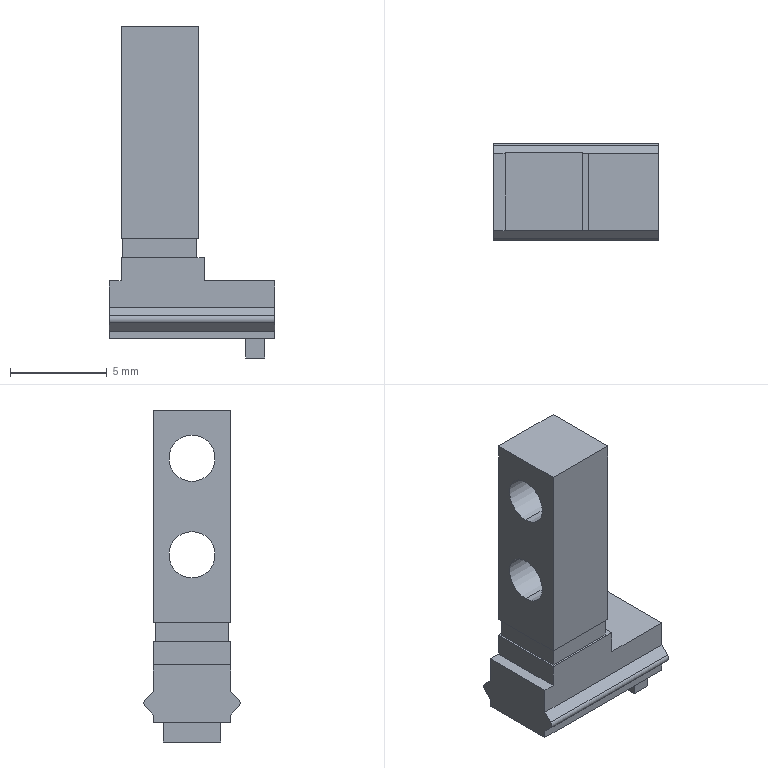Part | STEP file | MHZ2-6D2_Finger(0).stp | 1 solid | 37 faces | box 8.55 x 5 x 17.2 mm | volume 286.489 mm3 | plane 31 | cylinder 6 | commonest cylinder face diameters 2.4 x4 0.5 x2
STEP:
#1=CARTESIAN_POINT('',(-10.,0.,9.9));
#2=VERTEX_POINT('',#1);
#3=CARTESIAN_POINT('',(-10.,0.,7.5));
#4=VERTEX_POINT('',#3);
#5=CARTESIAN_POINT('',(-10.,0.,8.7));
#6=DIRECTION('',(1.,0.,0.));
#7=DIRECTION('',(0.,0.,-1.));
#8=AXIS2_PLACEMENT_3D('',#5,#6,#7);
#9=CIRCLE('',#8,1.2);
#10=EDGE_CURVE('',#2,#4,#9,.T.);
#11=ORIENTED_EDGE('',*,*,#10,.F.);
#12=CARTESIAN_POINT('',(-6.,0.,9.9));
#13=VERTEX_POINT('',#12);
#14=CARTESIAN_POINT('',(-6.,0.,9.9));
#15=DIRECTION('',(1.,0.,0.));
#16=VECTOR('',#15,1000.);
#17=LINE('',#14,#16);
#18=EDGE_CURVE('',#2,#13,#17,.T.);
#19=ORIENTED_EDGE('',*,*,#18,.T.);
#20=CARTESIAN_POINT('',(-6.,0.,7.5));
#21=VERTEX_POINT('',#20);
#22=CARTESIAN_POINT('',(-6.,0.,8.7));
#23=DIRECTION('',(1.,0.,0.));
#24=DIRECTION('',(0.,0.,-1.));
#25=AXIS2_PLACEMENT_3D('',#22,#23,#24);
#26=CIRCLE('',#25,1.2);
#27=EDGE_CURVE('',#13,#21,#26,.T.);
#28=ORIENTED_EDGE('',*,*,#27,.T.);
#29=CARTESIAN_POINT('',(-6.,0.,7.5));
#30=DIRECTION('',(1.,0.,0.));
#31=VECTOR('',#30,1000.);
#32=LINE('',#29,#31);
#33=EDGE_CURVE('',#4,#21,#32,.T.);
#34=ORIENTED_EDGE('',*,*,#33,.F.);
#35=EDGE_LOOP('',(#11,#19,#28,#34));
#36=FACE_OUTER_BOUND('',#35,.T.);
#37=CARTESIAN_POINT('',(-6.,0.,8.7));
#38=DIRECTION('',(1.,0.,0.));
#39=DIRECTION('',(0.,0.,-1.));
#40=AXIS2_PLACEMENT_3D('',#37,#38,#39);
#41=CYLINDRICAL_SURFACE('',#40,1.2);
#42=ADVANCED_FACE('',(#36),#41,.F.);
#43=CARTESIAN_POINT('',(-10.,0.,14.9));
#44=VERTEX_POINT('',#43);
#45=CARTESIAN_POINT('',(-10.,0.,12.5));
#46=VERTEX_POINT('',#45);
#47=CARTESIAN_POINT('',(-10.,0.,13.7));
#48=DIRECTION('',(1.,0.,0.));
#49=DIRECTION('',(0.,0.,-1.));
#50=AXIS2_PLACEMENT_3D('',#47,#48,#49);
#51=CIRCLE('',#50,1.2);
#52=EDGE_CURVE('',#44,#46,#51,.T.);
#53=ORIENTED_EDGE('',*,*,#52,.F.);
#54=CARTESIAN_POINT('',(-6.,0.,14.9));
#55=VERTEX_POINT('',#54);
#56=CARTESIAN_POINT('',(-6.,0.,14.9));
#57=DIRECTION('',(1.,0.,0.));
#58=VECTOR('',#57,1000.);
#59=LINE('',#56,#58);
#60=EDGE_CURVE('',#44,#55,#59,.T.);
#61=ORIENTED_EDGE('',*,*,#60,.T.);
#62=CARTESIAN_POINT('',(-6.,0.,12.5));
#63=VERTEX_POINT('',#62);
#64=CARTESIAN_POINT('',(-6.,0.,13.7));
#65=DIRECTION('',(1.,0.,0.));
#66=DIRECTION('',(0.,0.,-1.));
#67=AXIS2_PLACEMENT_3D('',#64,#65,#66);
#68=CIRCLE('',#67,1.2);
#69=EDGE_CURVE('',#55,#63,#68,.T.);
#70=ORIENTED_EDGE('',*,*,#69,.T.);
#71=CARTESIAN_POINT('',(-6.,0.,12.5));
#72=DIRECTION('',(1.,0.,0.));
#73=VECTOR('',#72,1000.);
#74=LINE('',#71,#73);
#75=EDGE_CURVE('',#46,#63,#74,.T.);
#76=ORIENTED_EDGE('',*,*,#75,.F.);
#77=EDGE_LOOP('',(#53,#61,#70,#76));
#78=FACE_OUTER_BOUND('',#77,.T.);
#79=CARTESIAN_POINT('',(-6.,0.,13.7));
#80=DIRECTION('',(1.,0.,0.));
#81=DIRECTION('',(0.,0.,-1.));
#82=AXIS2_PLACEMENT_3D('',#79,#80,#81);
#83=CYLINDRICAL_SURFACE('',#82,1.2);
#84=ADVANCED_FACE('',(#78),#83,.F.);
#85=CARTESIAN_POINT('',(-10.6,-2.,1.604));
#86=VERTEX_POINT('',#85);
#87=CARTESIAN_POINT('',(-10.6,-2.,3.));
#88=VERTEX_POINT('',#87);
#89=CARTESIAN_POINT('',(-10.6,-2.,0.));
#90=DIRECTION('',(0.,0.,1.));
#91=VECTOR('',#90,1000.);
#92=LINE('',#89,#91);
#93=EDGE_CURVE('',#86,#88,#92,.T.);
#94=ORIENTED_EDGE('',*,*,#93,.F.);
#95=CARTESIAN_POINT('',(-2.05,-2.,1.604));
#96=VERTEX_POINT('',#95);
#97=CARTESIAN_POINT('',(-10.6,-2.,1.604));
#98=DIRECTION('',(1.,0.,0.));
#99=VECTOR('',#98,1000.);
#100=LINE('',#97,#99);
#101=EDGE_CURVE('',#86,#96,#100,.T.);
#102=ORIENTED_EDGE('',*,*,#101,.T.);
#103=CARTESIAN_POINT('',(-2.05,-2.,3.));
#104=VERTEX_POINT('',#103);
#105=CARTESIAN_POINT('',(-2.05,-2.,3.));
#106=DIRECTION('',(0.,0.,-1.));
#107=VECTOR('',#106,1000.);
#108=LINE('',#105,#107);
#109=EDGE_CURVE('',#104,#96,#108,.T.);
#110=ORIENTED_EDGE('',*,*,#109,.F.);
#111=CARTESIAN_POINT('',(-5.7,-2.,3.));
#112=VERTEX_POINT('',#111);
#113=CARTESIAN_POINT('',(-5.7,-2.,3.));
#114=DIRECTION('',(1.,0.,0.));
#115=VECTOR('',#114,1000.);
#116=LINE('',#113,#115);
#117=EDGE_CURVE('',#112,#104,#116,.T.);
#118=ORIENTED_EDGE('',*,*,#117,.F.);
#119=CARTESIAN_POINT('',(-5.7,-2.,4.2));
#120=VERTEX_POINT('',#119);
#121=CARTESIAN_POINT('',(-5.7,-2.,4.2));
#122=DIRECTION('',(0.,0.,-1.));
#123=VECTOR('',#122,1000.);
#124=LINE('',#121,#123);
#125=EDGE_CURVE('',#120,#112,#124,.T.);
#126=ORIENTED_EDGE('',*,*,#125,.F.);
#127=CARTESIAN_POINT('',(-10.,-2.,4.2));
#128=VERTEX_POINT('',#127);
#129=CARTESIAN_POINT('',(-6.1,-2.,4.2));
#130=DIRECTION('',(1.,0.,0.));
#131=VECTOR('',#130,1000.);
#132=LINE('',#129,#131);
#133=EDGE_CURVE('',#128,#120,#132,.T.);
#134=ORIENTED_EDGE('',*,*,#133,.F.);
#135=CARTESIAN_POINT('',(-10.,-2.,3.));
#136=VERTEX_POINT('',#135);
#137=CARTESIAN_POINT('',(-10.,-2.,3.));
#138=DIRECTION('',(0.,0.,1.));
#139=VECTOR('',#138,1000.);
#140=LINE('',#137,#139);
#141=EDGE_CURVE('',#136,#128,#140,.T.);
#142=ORIENTED_EDGE('',*,*,#141,.F.);
#143=CARTESIAN_POINT('',(-10.6,-2.,3.));
#144=DIRECTION('',(1.,0.,0.));
#145=VECTOR('',#144,1000.);
#146=LINE('',#143,#145);
#147=EDGE_CURVE('',#88,#136,#146,.T.);
#148=ORIENTED_EDGE('',*,*,#147,.F.);
#149=EDGE_LOOP('',(#94,#102,#110,#118,#126,#134,#142,#148));
#150=FACE_OUTER_BOUND('',#149,.T.);
#151=CARTESIAN_POINT('',(0.,-2.,0.));
#152=DIRECTION('',(0.,1.,0.));
#153=DIRECTION('',(1.,0.,0.));
#154=AXIS2_PLACEMENT_3D('',#151,#152,#153);
#155=PLANE('',#154);
#156=ADVANCED_FACE('',(#150),#155,.F.);
#157=CARTESIAN_POINT('',(-10.6,2.,1.604));
#158=VERTEX_POINT('',#157);
#159=CARTESIAN_POINT('',(-2.05,2.,1.604));
#160=VERTEX_POINT('',#159);
#161=CARTESIAN_POINT('',(-10.6,2.,1.604));
#162=DIRECTION('',(1.,0.,0.));
#163=VECTOR('',#162,1000.);
#164=LINE('',#161,#163);
#165=EDGE_CURVE('',#158,#160,#164,.T.);
#166=ORIENTED_EDGE('',*,*,#165,.F.);
#167=CARTESIAN_POINT('',(-10.6,2.,3.));
#168=VERTEX_POINT('',#167);
#169=CARTESIAN_POINT('',(-10.6,2.,0.));
#170=DIRECTION('',(0.,0.,1.));
#171=VECTOR('',#170,1000.);
#172=LINE('',#169,#171);
#173=EDGE_CURVE('',#158,#168,#172,.T.);
#174=ORIENTED_EDGE('',*,*,#173,.T.);
#175=CARTESIAN_POINT('',(-10.,2.,3.));
#176=VERTEX_POINT('',#175);
#177=CARTESIAN_POINT('',(-10.6,2.,3.));
#178=DIRECTION('',(1.,0.,0.));
#179=VECTOR('',#178,1000.);
#180=LINE('',#177,#179);
#181=EDGE_CURVE('',#168,#176,#180,.T.);
#182=ORIENTED_EDGE('',*,*,#181,.T.);
#183=CARTESIAN_POINT('',(-10.,2.,4.2));
#184=VERTEX_POINT('',#183);
#185=CARTESIAN_POINT('',(-10.,2.,3.));
#186=DIRECTION('',(0.,0.,1.));
#187=VECTOR('',#186,1000.);
#188=LINE('',#185,#187);
#189=EDGE_CURVE('',#176,#184,#188,.T.);
#190=ORIENTED_EDGE('',*,*,#189,.T.);
#191=CARTESIAN_POINT('',(-5.7,2.,4.2));
#192=VERTEX_POINT('',#191);
#193=CARTESIAN_POINT('',(-10.,2.,4.2));
#194=DIRECTION('',(1.,0.,0.));
#195=VECTOR('',#194,1000.);
#196=LINE('',#193,#195);
#197=EDGE_CURVE('',#184,#192,#196,.T.);
#198=ORIENTED_EDGE('',*,*,#197,.T.);
#199=CARTESIAN_POINT('',(-5.7,2.,3.));
#200=VERTEX_POINT('',#199);
#201=CARTESIAN_POINT('',(-5.7,2.,4.2));
#202=DIRECTION('',(0.,0.,-1.));
#203=VECTOR('',#202,1000.);
#204=LINE('',#201,#203);
#205=EDGE_CURVE('',#192,#200,#204,.T.);
#206=ORIENTED_EDGE('',*,*,#205,.T.);
#207=CARTESIAN_POINT('',(-2.05,2.,3.));
#208=VERTEX_POINT('',#207);
#209=CARTESIAN_POINT('',(-5.7,2.,3.));
#210=DIRECTION('',(1.,0.,0.));
#211=VECTOR('',#210,1000.);
#212=LINE('',#209,#211);
#213=EDGE_CURVE('',#200,#208,#212,.T.);
#214=ORIENTED_EDGE('',*,*,#213,.T.);
#215=CARTESIAN_POINT('',(-2.05,2.,3.));
#216=DIRECTION('',(0.,0.,-1.));
#217=VECTOR('',#216,1000.);
#218=LINE('',#215,#217);
#219=EDGE_CURVE('',#208,#160,#218,.T.);
#220=ORIENTED_EDGE('',*,*,#219,.T.);
#221=EDGE_LOOP('',(#166,#174,#182,#190,#198,#206,#214,#220));
#222=FACE_OUTER_BOUND('',#221,.T.);
#223=CARTESIAN_POINT('',(0.,2.,0.));
#224=DIRECTION('',(0.,1.,0.));
#225=DIRECTION('',(1.,0.,0.));
#226=AXIS2_PLACEMENT_3D('',#223,#224,#225);
#227=PLANE('',#226);
#228=ADVANCED_FACE('',(#222),#227,.T.);
#229=CARTESIAN_POINT('',(-2.05,-2.,0.));
#230=VERTEX_POINT('',#229);
#231=CARTESIAN_POINT('',(-10.6,-2.,0.));
#232=VERTEX_POINT('',#231);
#233=CARTESIAN_POINT('',(-2.05,-2.,0.));
#234=DIRECTION('',(-1.,0.,0.));
#235=VECTOR('',#234,1000.);
#236=LINE('',#233,#235);
#237=EDGE_CURVE('',#230,#232,#236,.T.);
#238=ORIENTED_EDGE('',*,*,#237,.T.);
#239=CARTESIAN_POINT('',(-10.6,2.,0.));
#240=VERTEX_POINT('',#239);
#241=CARTESIAN_POINT('',(-10.6,2.,0.));
#242=DIRECTION('',(0.,-1.,0.));
#243=VECTOR('',#242,1000.);
#244=LINE('',#241,#243);
#245=EDGE_CURVE('',#240,#232,#244,.T.);
#246=ORIENTED_EDGE('',*,*,#245,.F.);
#247=CARTESIAN_POINT('',(-2.05,2.,0.));
#248=VERTEX_POINT('',#247);
#249=CARTESIAN_POINT('',(-2.05,2.,0.));
#250=DIRECTION('',(-1.,0.,0.));
#251=VECTOR('',#250,1000.);
#252=LINE('',#249,#251);
#253=EDGE_CURVE('',#248,#240,#252,.T.);
#254=ORIENTED_EDGE('',*,*,#253,.F.);
#255=CARTESIAN_POINT('',(-2.05,2.,0.));
#256=DIRECTION('',(0.,-1.,0.));
#257=VECTOR('',#256,1000.);
#258=LINE('',#255,#257);
#259=EDGE_CURVE('',#248,#230,#258,.T.);
#260=ORIENTED_EDGE('',*,*,#259,.T.);
#261=EDGE_LOOP('',(#238,#246,#254,#260));
#262=FACE_OUTER_BOUND('',#261,.T.);
#263=CARTESIAN_POINT('',(-3.55,1.5,0.));
#264=VERTEX_POINT('',#263);
#265=CARTESIAN_POINT('',(-3.55,-1.5,0.));
#266=VERTEX_POINT('',#265);
#267=CARTESIAN_POINT('',(-3.55,1.5,0.));
#268=DIRECTION('',(0.,-1.,0.));
#269=VECTOR('',#268,1000.);
#270=LINE('',#267,#269);
#271=EDGE_CURVE('',#264,#266,#270,.T.);
#272=ORIENTED_EDGE('',*,*,#271,.T.);
#273=CARTESIAN_POINT('',(-2.55,-1.5,0.));
#274=VERTEX_POINT('',#273);
#275=CARTESIAN_POINT('',(-3.55,-1.5,0.));
#276=DIRECTION('',(1.,0.,0.));
#277=VECTOR('',#276,1000.);
#278=LINE('',#275,#277);
#279=EDGE_CURVE('',#266,#274,#278,.T.);
#280=ORIENTED_EDGE('',*,*,#279,.T.);
#281=CARTESIAN_POINT('',(-2.55,1.5,0.));
#282=VERTEX_POINT('',#281);
#283=CARTESIAN_POINT('',(-2.55,1.5,0.));
#284=DIRECTION('',(0.,-1.,0.));
#285=VECTOR('',#284,1000.);
#286=LINE('',#283,#285);
#287=EDGE_CURVE('',#282,#274,#286,.T.);
#288=ORIENTED_EDGE('',*,*,#287,.F.);
#289=CARTESIAN_POINT('',(-3.55,1.5,0.));
#290=DIRECTION('',(1.,0.,0.));
#291=VECTOR('',#290,1000.);
#292=LINE('',#289,#291);
#293=EDGE_CURVE('',#264,#282,#292,.T.);
#294=ORIENTED_EDGE('',*,*,#293,.F.);
#295=EDGE_LOOP('',(#272,#280,#288,#294));
#296=FACE_BOUND('',#295,.T.);
#297=CARTESIAN_POINT('',(-2.05,2.,0.));
#298=DIRECTION('',(0.,0.,1.));
#299=DIRECTION('',(1.,0.,0.));
#300=AXIS2_PLACEMENT_3D('',#297,#298,#299);
#301=PLANE('',#300);
#302=ADVANCED_FACE('',(#262,#296),#301,.F.);
#303=CARTESIAN_POINT('',(-9.9,-1.9,5.2));
#304=VERTEX_POINT('',#303);
#305=CARTESIAN_POINT('',(-9.9,-1.9,4.2));
#306=VERTEX_POINT('',#305);
#307=CARTESIAN_POINT('',(-9.9,-1.9,4.2));
#308=DIRECTION('',(0.,0.,-1.));
#309=VECTOR('',#308,1000.);
#310=LINE('',#307,#309);
#311=EDGE_CURVE('',#304,#306,#310,.T.);
#312=ORIENTED_EDGE('',*,*,#311,.F.);
#313=CARTESIAN_POINT('',(-9.9,1.9,5.2));
#314=VERTEX_POINT('',#313);
#315=CARTESIAN_POINT('',(-9.9,2.,5.2));
#316=DIRECTION('',(0.,-1.,0.));
#317=VECTOR('',#316,1000.);
#318=LINE('',#315,#317);
#319=EDGE_CURVE('',#314,#304,#318,.T.);
#320=ORIENTED_EDGE('',*,*,#319,.F.);
#321=CARTESIAN_POINT('',(-9.9,1.9,4.2));
#322=VERTEX_POINT('',#321);
#323=CARTESIAN_POINT('',(-9.9,1.9,4.2));
#324=DIRECTION('',(0.,0.,1.));
#325=VECTOR('',#324,1000.);
#326=LINE('',#323,#325);
#327=EDGE_CURVE('',#322,#314,#326,.T.);
#328=ORIENTED_EDGE('',*,*,#327,.F.);
#329=CARTESIAN_POINT('',(-9.9,2.,4.2));
#330=DIRECTION('',(0.,-1.,0.));
#331=VECTOR('',#330,1000.);
#332=LINE('',#329,#331);
#333=EDGE_CURVE('',#322,#306,#332,.T.);
#334=ORIENTED_EDGE('',*,*,#333,.T.);
#335=EDGE_LOOP('',(#312,#320,#328,#334));
#336=FACE_OUTER_BOUND('',#335,.T.);
#337=CARTESIAN_POINT('',(-9.9,2.,4.2));
#338=DIRECTION('',(1.,0.,0.));
#339=DIRECTION('',(0.,1.,0.));
#340=AXIS2_PLACEMENT_3D('',#337,#338,#339);
#341=PLANE('',#340);
#342=ADVANCED_FACE('',(#336),#341,.F.);
#343=CARTESIAN_POINT('',(-6.1,-1.9,4.2));
#344=VERTEX_POINT('',#343);
#345=CARTESIAN_POINT('',(-6.1,-1.9,5.2));
#346=VERTEX_POINT('',#345);
#347=CARTESIAN_POINT('',(-6.1,-1.9,5.2));
#348=DIRECTION('',(0.,0.,1.));
#349=VECTOR('',#348,1000.);
#350=LINE('',#347,#349);
#351=EDGE_CURVE('',#344,#346,#350,.T.);
#352=ORIENTED_EDGE('',*,*,#351,.F.);
#353=CARTESIAN_POINT('',(-6.1,1.9,4.2));
#354=VERTEX_POINT('',#353);
#355=CARTESIAN_POINT('',(-6.1,2.,4.2));
#356=DIRECTION('',(0.,-1.,0.));
#357=VECTOR('',#356,1000.);
#358=LINE('',#355,#357);
#359=EDGE_CURVE('',#354,#344,#358,.T.);
#360=ORIENTED_EDGE('',*,*,#359,.F.);
#361=CARTESIAN_POINT('',(-6.1,1.9,5.2));
#362=VERTEX_POINT('',#361);
#363=CARTESIAN_POINT('',(-6.1,1.9,5.2));
#364=DIRECTION('',(0.,0.,-1.));
#365=VECTOR('',#364,1000.);
#366=LINE('',#363,#365);
#367=EDGE_CURVE('',#362,#354,#366,.T.);
#368=ORIENTED_EDGE('',*,*,#367,.F.);
#369=CARTESIAN_POINT('',(-6.1,2.,5.2));
#370=DIRECTION('',(0.,-1.,0.));
#371=VECTOR('',#370,1000.);
#372=LINE('',#369,#371);
#373=EDGE_CURVE('',#362,#346,#372,.T.);
#374=ORIENTED_EDGE('',*,*,#373,.T.);
#375=EDGE_LOOP('',(#352,#360,#368,#374));
#376=FACE_OUTER_BOUND('',#375,.T.);
#377=CARTESIAN_POINT('',(-6.1,2.,5.2));
#378=DIRECTION('',(-1.,0.,0.));
#379=DIRECTION('',(0.,0.,1.));
#380=AXIS2_PLACEMENT_3D('',#377,#378,#379);
#381=PLANE('',#380);
#382=ADVANCED_FACE('',(#376),#381,.F.);
#383=CARTESIAN_POINT('',(-10.,-2.,5.2));
#384=VERTEX_POINT('',#383);
#385=CARTESIAN_POINT('',(-10.,-2.,16.2));
#386=VERTEX_POINT('',#385);
#387=CARTESIAN_POINT('',(-10.,-2.,5.2));
#388=DIRECTION('',(0.,0.,1.));
#389=VECTOR('',#388,1000.);
#390=LINE('',#387,#389);
#391=EDGE_CURVE('',#384,#386,#390,.T.);
#392=ORIENTED_EDGE('',*,*,#391,.F.);
#393=CARTESIAN_POINT('',(-6.,-2.,5.2));
#394=VERTEX_POINT('',#393);
#395=CARTESIAN_POINT('',(-6.,-2.,5.2));
#396=DIRECTION('',(-1.,0.,0.));
#397=VECTOR('',#396,1000.);
#398=LINE('',#395,#397);
#399=EDGE_CURVE('',#394,#384,#398,.T.);
#400=ORIENTED_EDGE('',*,*,#399,.F.);
#401=CARTESIAN_POINT('',(-6.,-2.,16.2));
#402=VERTEX_POINT('',#401);
#403=CARTESIAN_POINT('',(-6.,-2.,16.2));
#404=DIRECTION('',(0.,0.,-1.));
#405=VECTOR('',#404,1000.);
#406=LINE('',#403,#405);
#407=EDGE_CURVE('',#402,#394,#406,.T.);
#408=ORIENTED_EDGE('',*,*,#407,.F.);
#409=CARTESIAN_POINT('',(-10.,-2.,16.2));
#410=DIRECTION('',(1.,0.,0.));
#411=VECTOR('',#410,1000.);
#412=LINE('',#409,#411);
#413=EDGE_CURVE('',#386,#402,#412,.T.);
#414=ORIENTED_EDGE('',*,*,#413,.F.);
#415=EDGE_LOOP('',(#392,#400,#408,#414));
#416=FACE_OUTER_BOUND('',#415,.T.);
#417=CARTESIAN_POINT('',(0.,-2.,0.));
#418=DIRECTION('',(0.,1.,0.));
#419=DIRECTION('',(1.,0.,0.));
#420=AXIS2_PLACEMENT_3D('',#417,#418,#419);
#421=PLANE('',#420);
#422=ADVANCED_FACE('',(#416),#421,.F.);
#423=CARTESIAN_POINT('',(-2.05,-2.,0.3964));
#424=VERTEX_POINT('',#423);
#425=CARTESIAN_POINT('',(-2.05,-2.,3.));
#426=DIRECTION('',(0.,0.,-1.));
#427=VECTOR('',#426,1000.);
#428=LINE('',#425,#427);
#429=EDGE_CURVE('',#424,#230,#428,.T.);
#430=ORIENTED_EDGE('',*,*,#429,.F.);
#431=CARTESIAN_POINT('',(-10.6,-2.,0.3964));
#432=VERTEX_POINT('',#431);
#433=CARTESIAN_POINT('',(-10.6,-2.,0.3964));
#434=DIRECTION('',(1.,0.,0.));
#435=VECTOR('',#434,1000.);
#436=LINE('',#433,#435);
#437=EDGE_CURVE('',#432,#424,#436,.T.);
#438=ORIENTED_EDGE('',*,*,#437,.F.);
#439=CARTESIAN_POINT('',(-10.6,-2.,0.));
#440=DIRECTION('',(0.,0.,1.));
#441=VECTOR('',#440,1000.);
#442=LINE('',#439,#441);
#443=EDGE_CURVE('',#232,#432,#442,.T.);
#444=ORIENTED_EDGE('',*,*,#443,.F.);
#445=ORIENTED_EDGE('',*,*,#237,.F.);
#446=EDGE_LOOP('',(#430,#438,#444,#445));
#447=FACE_OUTER_BOUND('',#446,.T.);
#448=CARTESIAN_POINT('',(0.,-2.,0.));
#449=DIRECTION('',(0.,1.,0.));
#450=DIRECTION('',(1.,0.,0.));
#451=AXIS2_PLACEMENT_3D('',#448,#449,#450);
#452=PLANE('',#451);
#453=ADVANCED_FACE('',(#447),#452,.F.);
#454=CARTESIAN_POINT('',(-6.,2.,16.2));
#455=VERTEX_POINT('',#454);
#456=CARTESIAN_POINT('',(-6.,2.,5.2));
#457=VERTEX_POINT('',#456);
#458=CARTESIAN_POINT('',(-6.,2.,16.2));
#459=DIRECTION('',(0.,0.,-1.));
#460=VECTOR('',#459,1000.);
#461=LINE('',#458,#460);
#462=EDGE_CURVE('',#455,#457,#461,.T.);
#463=ORIENTED_EDGE('',*,*,#462,.T.);
#464=CARTESIAN_POINT('',(-10.,2.,5.2));
#465=VERTEX_POINT('',#464);
#466=CARTESIAN_POINT('',(-9.9,2.,5.2));
#467=DIRECTION('',(-1.,0.,0.));
#468=VECTOR('',#467,1000.);
#469=LINE('',#466,#468);
#470=EDGE_CURVE('',#457,#465,#469,.T.);
#471=ORIENTED_EDGE('',*,*,#470,.T.);
#472=CARTESIAN_POINT('',(-10.,2.,16.2));
#473=VERTEX_POINT('',#472);
#474=CARTESIAN_POINT('',(-10.,2.,5.2));
#475=DIRECTION('',(0.,0.,1.));
#476=VECTOR('',#475,1000.);
#477=LINE('',#474,#476);
#478=EDGE_CURVE('',#465,#473,#477,.T.);
#479=ORIENTED_EDGE('',*,*,#478,.T.);
#480=CARTESIAN_POINT('',(-10.,2.,16.2));
#481=DIRECTION('',(1.,0.,0.));
#482=VECTOR('',#481,1000.);
#483=LINE('',#480,#482);
#484=EDGE_CURVE('',#473,#455,#483,.T.);
#485=ORIENTED_EDGE('',*,*,#484,.T.);
#486=EDGE_LOOP('',(#463,#471,#479,#485));
#487=FACE_OUTER_BOUND('',#486,.T.);
#488=CARTESIAN_POINT('',(0.,2.,0.));
#489=DIRECTION('',(0.,1.,0.));
#490=DIRECTION('',(1.,0.,0.));
#491=AXIS2_PLACEMENT_3D('',#488,#489,#490);
#492=PLANE('',#491);
#493=ADVANCED_FACE('',(#487),#492,.T.);
#494=CARTESIAN_POINT('',(-10.6,2.,0.3964));
#495=VERTEX_POINT('',#494);
#496=CARTESIAN_POINT('',(-2.05,2.,0.3964));
#497=VERTEX_POINT('',#496);
#498=CARTESIAN_POINT('',(-10.6,2.,0.3964));
#499=DIRECTION('',(1.,0.,0.));
#500=VECTOR('',#499,1000.);
#501=LINE('',#498,#500);
#502=EDGE_CURVE('',#495,#497,#501,.T.);
#503=ORIENTED_EDGE('',*,*,#502,.T.);
#504=CARTESIAN_POINT('',(-2.05,2.,3.));
#505=DIRECTION('',(0.,0.,-1.));
#506=VECTOR('',#505,1000.);
#507=LINE('',#504,#506);
#508=EDGE_CURVE('',#497,#248,#507,.T.);
#509=ORIENTED_EDGE('',*,*,#508,.T.);
#510=ORIENTED_EDGE('',*,*,#253,.T.);
#511=CARTESIAN_POINT('',(-10.6,2.,0.));
#512=DIRECTION('',(0.,0.,1.));
#513=VECTOR('',#512,1000.);
#514=LINE('',#511,#513);
#515=EDGE_CURVE('',#240,#495,#514,.T.);
#516=ORIENTED_EDGE('',*,*,#515,.T.);
#517=EDGE_LOOP('',(#503,#509,#510,#516));
#518=FACE_OUTER_BOUND('',#517,.T.);
#519=CARTESIAN_POINT('',(0.,2.,0.));
#520=DIRECTION('',(0.,1.,0.));
#521=DIRECTION('',(1.,0.,0.));
#522=AXIS2_PLACEMENT_3D('',#519,#520,#521);
#523=PLANE('',#522);
#524=ADVANCED_FACE('',(#518),#523,.T.);
#525=ORIENTED_EDGE('',*,*,#443,.T.);
#526=CARTESIAN_POINT('',(-10.6,-2.427,0.8232));
#527=VERTEX_POINT('',#526);
#528=CARTESIAN_POINT('',(-10.6,-2.427,0.8232));
#529=DIRECTION('',(0.,0.7071,-0.7071));
#530=VECTOR('',#529,1000.);
#531=LINE('',#528,#530);
#532=EDGE_CURVE('',#527,#432,#531,.T.);
#533=ORIENTED_EDGE('',*,*,#532,.F.);
#534=CARTESIAN_POINT('',(-10.6,-2.427,1.177));
#535=VERTEX_POINT('',#534);
#536=CARTESIAN_POINT('',(-10.6,-2.25,1.));
#537=DIRECTION('',(1.,0.,0.));
#538=DIRECTION('',(0.,0.,-1.));
#539=AXIS2_PLACEMENT_3D('',#536,#537,#538);
#540=CIRCLE('',#539,0.25);
#541=EDGE_CURVE('',#535,#527,#540,.T.);
#542=ORIENTED_EDGE('',*,*,#541,.F.);
#543=CARTESIAN_POINT('',(-10.6,-2.,1.604));
#544=DIRECTION('',(0.,-0.7071,-0.7071));
#545=VECTOR('',#544,1000.);
#546=LINE('',#543,#545);
#547=EDGE_CURVE('',#86,#535,#546,.T.);
#548=ORIENTED_EDGE('',*,*,#547,.F.);
#549=ORIENTED_EDGE('',*,*,#93,.T.);
#550=CARTESIAN_POINT('',(-10.6,2.,3.));
#551=DIRECTION('',(0.,-1.,0.));
#552=VECTOR('',#551,1000.);
#553=LINE('',#550,#552);
#554=EDGE_CURVE('',#168,#88,#553,.T.);
#555=ORIENTED_EDGE('',*,*,#554,.F.);
#556=ORIENTED_EDGE('',*,*,#173,.F.);
#557=CARTESIAN_POINT('',(-10.6,2.427,1.177));
#558=VERTEX_POINT('',#557);
#559=CARTESIAN_POINT('',(-10.6,2.427,1.177));
#560=DIRECTION('',(0.,-0.7071,0.7071));
#561=VECTOR('',#560,1000.);
#562=LINE('',#559,#561);
#563=EDGE_CURVE('',#558,#158,#562,.T.);
#564=ORIENTED_EDGE('',*,*,#563,.F.);
#565=CARTESIAN_POINT('',(-10.6,2.427,0.8232));
#566=VERTEX_POINT('',#565);
#567=CARTESIAN_POINT('',(-10.6,2.25,1.));
#568=DIRECTION('',(1.,0.,0.));
#569=DIRECTION('',(0.,0.,-1.));
#570=AXIS2_PLACEMENT_3D('',#567,#568,#569);
#571=CIRCLE('',#570,0.25);
#572=EDGE_CURVE('',#566,#558,#571,.T.);
#573=ORIENTED_EDGE('',*,*,#572,.F.);
#574=CARTESIAN_POINT('',(-10.6,2.,0.3964));
#575=DIRECTION('',(0.,0.7071,0.7071));
#576=VECTOR('',#575,1000.);
#577=LINE('',#574,#576);
#578=EDGE_CURVE('',#495,#566,#577,.T.);
#579=ORIENTED_EDGE('',*,*,#578,.F.);
#580=ORIENTED_EDGE('',*,*,#515,.F.);
#581=ORIENTED_EDGE('',*,*,#245,.T.);
#582=EDGE_LOOP('',(#525,#533,#542,#548,#549,#555,#556,#564,#573,#579,#580,#581));
#583=FACE_OUTER_BOUND('',#582,.T.);
#584=CARTESIAN_POINT('',(-10.6,2.,0.));
#585=DIRECTION('',(1.,0.,0.));
#586=DIRECTION('',(0.,1.,0.));
#587=AXIS2_PLACEMENT_3D('',#584,#585,#586);
#588=PLANE('',#587);
#589=ADVANCED_FACE('',(#583),#588,.F.);
#590=ORIENTED_EDGE('',*,*,#147,.T.);
#591=CARTESIAN_POINT('',(-10.,2.,3.));
#592=DIRECTION('',(0.,-1.,0.));
#593=VECTOR('',#592,1000.);
#594=LINE('',#591,#593);
#595=EDGE_CURVE('',#176,#136,#594,.T.);
#596=ORIENTED_EDGE('',*,*,#595,.F.);
#597=ORIENTED_EDGE('',*,*,#181,.F.);
#598=ORIENTED_EDGE('',*,*,#554,.T.);
#599=EDGE_LOOP('',(#590,#596,#597,#598));
#600=FACE_OUTER_BOUND('',#599,.T.);
#601=CARTESIAN_POINT('',(-10.6,2.,3.));
#602=DIRECTION('',(0.,0.,-1.));
#603=DIRECTION('',(0.,-1.,0.));
#604=AXIS2_PLACEMENT_3D('',#601,#602,#603);
#605=PLANE('',#604);
#606=ADVANCED_FACE('',(#600),#605,.F.);
#607=ORIENTED_EDGE('',*,*,#141,.T.);
#608=CARTESIAN_POINT('',(-10.,2.,4.2));
#609=DIRECTION('',(0.,-1.,0.));
#610=VECTOR('',#609,1000.);
#611=LINE('',#608,#610);
#612=EDGE_CURVE('',#184,#128,#611,.T.);
#613=ORIENTED_EDGE('',*,*,#612,.F.);
#614=ORIENTED_EDGE('',*,*,#189,.F.);
#615=ORIENTED_EDGE('',*,*,#595,.T.);
#616=EDGE_LOOP('',(#607,#613,#614,#615));
#617=FACE_OUTER_BOUND('',#616,.T.);
#618=CARTESIAN_POINT('',(-10.,2.,3.));
#619=DIRECTION('',(1.,0.,0.));
#620=DIRECTION('',(0.,1.,0.));
#621=AXIS2_PLACEMENT_3D('',#618,#619,#620);
#622=PLANE('',#621);
#623=ADVANCED_FACE('',(#617),#622,.F.);
#624=CARTESIAN_POINT('',(-10.,0.,8.7));
#625=DIRECTION('',(1.,0.,0.));
#626=DIRECTION('',(0.,0.,-1.));
#627=AXIS2_PLACEMENT_3D('',#624,#625,#626);
#628=CIRCLE('',#627,1.2);
#629=EDGE_CURVE('',#4,#2,#628,.T.);
#630=ORIENTED_EDGE('',*,*,#629,.T.);
#631=ORIENTED_EDGE('',*,*,#10,.T.);
#632=EDGE_LOOP('',(#630,#631));
#633=FACE_BOUND('',#632,.T.);
#634=CARTESIAN_POINT('',(-10.,0.,13.7));
#635=DIRECTION('',(1.,0.,0.));
#636=DIRECTION('',(0.,0.,-1.));
#637=AXIS2_PLACEMENT_3D('',#634,#635,#636);
#638=CIRCLE('',#637,1.2);
#639=EDGE_CURVE('',#46,#44,#638,.T.);
#640=ORIENTED_EDGE('',*,*,#639,.T.);
#641=ORIENTED_EDGE('',*,*,#52,.T.);
#642=EDGE_LOOP('',(#640,#641));
#643=FACE_BOUND('',#642,.T.);
#644=ORIENTED_EDGE('',*,*,#391,.T.);
#645=CARTESIAN_POINT('',(-10.,2.,16.2));
#646=DIRECTION('',(0.,-1.,0.));
#647=VECTOR('',#646,1000.);
#648=LINE('',#645,#647);
#649=EDGE_CURVE('',#473,#386,#648,.T.);
#650=ORIENTED_EDGE('',*,*,#649,.F.);
#651=ORIENTED_EDGE('',*,*,#478,.F.);
#652=CARTESIAN_POINT('',(-10.,2.,5.2));
#653=DIRECTION('',(0.,-1.,0.));
#654=VECTOR('',#653,1000.);
#655=LINE('',#652,#654);
#656=EDGE_CURVE('',#465,#384,#655,.T.);
#657=ORIENTED_EDGE('',*,*,#656,.T.);
#658=EDGE_LOOP('',(#644,#650,#651,#657));
#659=FACE_OUTER_BOUND('',#658,.T.);
#660=CARTESIAN_POINT('',(-10.,2.,5.2));
#661=DIRECTION('',(1.,0.,0.));
#662=DIRECTION('',(0.,1.,0.));
#663=AXIS2_PLACEMENT_3D('',#660,#661,#662);
#664=PLANE('',#663);
#665=ADVANCED_FACE('',(#633,#643,#659),#664,.F.);
#666=ORIENTED_EDGE('',*,*,#413,.T.);
#667=CARTESIAN_POINT('',(-6.,2.,16.2));
#668=DIRECTION('',(0.,-1.,0.));
#669=VECTOR('',#668,1000.);
#670=LINE('',#667,#669);
#671=EDGE_CURVE('',#455,#402,#670,.T.);
#672=ORIENTED_EDGE('',*,*,#671,.F.);
#673=ORIENTED_EDGE('',*,*,#484,.F.);
#674=ORIENTED_EDGE('',*,*,#649,.T.);
#675=EDGE_LOOP('',(#666,#672,#673,#674));
#676=FACE_OUTER_BOUND('',#675,.T.);
#677=CARTESIAN_POINT('',(-10.,2.,16.2));
#678=DIRECTION('',(0.,0.,-1.));
#679=DIRECTION('',(-1.,0.,0.));
#680=AXIS2_PLACEMENT_3D('',#677,#678,#679);
#681=PLANE('',#680);
#682=ADVANCED_FACE('',(#676),#681,.F.);
#683=CARTESIAN_POINT('',(-6.,0.,8.7));
#684=DIRECTION('',(1.,0.,0.));
#685=DIRECTION('',(0.,0.,-1.));
#686=AXIS2_PLACEMENT_3D('',#683,#684,#685);
#687=CIRCLE('',#686,1.2);
#688=EDGE_CURVE('',#21,#13,#687,.T.);
#689=ORIENTED_EDGE('',*,*,#688,.F.);
#690=ORIENTED_EDGE('',*,*,#27,.F.);
#691=EDGE_LOOP('',(#689,#690));
#692=FACE_BOUND('',#691,.T.);
#693=CARTESIAN_POINT('',(-6.,0.,13.7));
#694=DIRECTION('',(1.,0.,0.));
#695=DIRECTION('',(0.,0.,-1.));
#696=AXIS2_PLACEMENT_3D('',#693,#694,#695);
#697=CIRCLE('',#696,1.2);
#698=EDGE_CURVE('',#63,#55,#697,.T.);
#699=ORIENTED_EDGE('',*,*,#698,.F.);
#700=ORIENTED_EDGE('',*,*,#69,.F.);
#701=EDGE_LOOP('',(#699,#700));
#702=FACE_BOUND('',#701,.T.);
#703=ORIENTED_EDGE('',*,*,#407,.T.);
#704=CARTESIAN_POINT('',(-6.,2.,5.2));
#705=DIRECTION('',(0.,-1.,0.));
#706=VECTOR('',#705,1000.);
#707=LINE('',#704,#706);
#708=EDGE_CURVE('',#457,#394,#707,.T.);
#709=ORIENTED_EDGE('',*,*,#708,.F.);
#710=ORIENTED_EDGE('',*,*,#462,.F.);
#711=ORIENTED_EDGE('',*,*,#671,.T.);
#712=EDGE_LOOP('',(#703,#709,#710,#711));
#713=FACE_OUTER_BOUND('',#712,.T.);
#714=CARTESIAN_POINT('',(-6.,2.,16.2));
#715=DIRECTION('',(-1.,0.,0.));
#716=DIRECTION('',(0.,0.,1.));
#717=AXIS2_PLACEMENT_3D('',#714,#715,#716);
#718=PLANE('',#717);
#719=ADVANCED_FACE('',(#692,#702,#713),#718,.F.);
#720=ORIENTED_EDGE('',*,*,#319,.T.);
#721=CARTESIAN_POINT('',(-6.,-1.9,5.2));
#722=DIRECTION('',(-1.,0.,0.));
#723=VECTOR('',#722,1000.);
#724=LINE('',#721,#723);
#725=EDGE_CURVE('',#346,#304,#724,.T.);
#726=ORIENTED_EDGE('',*,*,#725,.F.);
#727=ORIENTED_EDGE('',*,*,#373,.F.);
#728=CARTESIAN_POINT('',(-6.,1.9,5.2));
#729=DIRECTION('',(-1.,0.,0.));
#730=VECTOR('',#729,1000.);
#731=LINE('',#728,#730);
#732=EDGE_CURVE('',#362,#314,#731,.T.);
#733=ORIENTED_EDGE('',*,*,#732,.T.);
#734=EDGE_LOOP('',(#720,#726,#727,#733));
#735=FACE_BOUND('',#734,.T.);
#736=ORIENTED_EDGE('',*,*,#399,.T.);
#737=ORIENTED_EDGE('',*,*,#656,.F.);
#738=ORIENTED_EDGE('',*,*,#470,.F.);
#739=ORIENTED_EDGE('',*,*,#708,.T.);
#740=EDGE_LOOP('',(#736,#737,#738,#739));
#741=FACE_OUTER_BOUND('',#740,.T.);
#742=CARTESIAN_POINT('',(-6.,2.,5.2));
#743=DIRECTION('',(0.,0.,1.));
#744=DIRECTION('',(1.,0.,0.));
#745=AXIS2_PLACEMENT_3D('',#742,#743,#744);
#746=PLANE('',#745);
#747=ADVANCED_FACE('',(#735,#741),#746,.F.);
#748=ORIENTED_EDGE('',*,*,#612,.T.);
#749=ORIENTED_EDGE('',*,*,#133,.T.);
#750=CARTESIAN_POINT('',(-5.7,2.,4.2));
#751=DIRECTION('',(0.,-1.,0.));
#752=VECTOR('',#751,1000.);
#753=LINE('',#750,#752);
#754=EDGE_CURVE('',#192,#120,#753,.T.);
#755=ORIENTED_EDGE('',*,*,#754,.F.);
#756=ORIENTED_EDGE('',*,*,#197,.F.);
#757=EDGE_LOOP('',(#748,#749,#755,#756));
#758=FACE_OUTER_BOUND('',#757,.T.);
#759=ORIENTED_EDGE('',*,*,#359,.T.);
#760=CARTESIAN_POINT('',(-6.,-1.9,4.2));
#761=DIRECTION('',(-1.,0.,0.));
#762=VECTOR('',#761,1000.);
#763=LINE('',#760,#762);
#764=EDGE_CURVE('',#344,#306,#763,.T.);
#765=ORIENTED_EDGE('',*,*,#764,.T.);
#766=ORIENTED_EDGE('',*,*,#333,.F.);
#767=CARTESIAN_POINT('',(-6.,1.9,4.2));
#768=DIRECTION('',(-1.,0.,0.));
#769=VECTOR('',#768,1000.);
#770=LINE('',#767,#769);
#771=EDGE_CURVE('',#354,#322,#770,.T.);
#772=ORIENTED_EDGE('',*,*,#771,.F.);
#773=EDGE_LOOP('',(#759,#765,#766,#772));
#774=FACE_BOUND('',#773,.T.);
#775=CARTESIAN_POINT('',(-6.1,2.,4.2));
#776=DIRECTION('',(0.,0.,-1.));
#777=DIRECTION('',(0.,-1.,0.));
#778=AXIS2_PLACEMENT_3D('',#775,#776,#777);
#779=PLANE('',#778);
#780=ADVANCED_FACE('',(#758,#774),#779,.F.);
#781=ORIENTED_EDGE('',*,*,#125,.T.);
#782=CARTESIAN_POINT('',(-5.7,2.,3.));
#783=DIRECTION('',(0.,-1.,0.));
#784=VECTOR('',#783,1000.);
#785=LINE('',#782,#784);
#786=EDGE_CURVE('',#200,#112,#785,.T.);
#787=ORIENTED_EDGE('',*,*,#786,.F.);
#788=ORIENTED_EDGE('',*,*,#205,.F.);
#789=ORIENTED_EDGE('',*,*,#754,.T.);
#790=EDGE_LOOP('',(#781,#787,#788,#789));
#791=FACE_OUTER_BOUND('',#790,.T.);
#792=CARTESIAN_POINT('',(-5.7,2.,4.2));
#793=DIRECTION('',(-1.,0.,0.));
#794=DIRECTION('',(0.,0.,1.));
#795=AXIS2_PLACEMENT_3D('',#792,#793,#794);
#796=PLANE('',#795);
#797=ADVANCED_FACE('',(#791),#796,.F.);
#798=ORIENTED_EDGE('',*,*,#117,.T.);
#799=CARTESIAN_POINT('',(-2.05,2.,3.));
#800=DIRECTION('',(0.,-1.,0.));
#801=VECTOR('',#800,1000.);
#802=LINE('',#799,#801);
#803=EDGE_CURVE('',#208,#104,#802,.T.);
#804=ORIENTED_EDGE('',*,*,#803,.F.);
#805=ORIENTED_EDGE('',*,*,#213,.F.);
#806=ORIENTED_EDGE('',*,*,#786,.T.);
#807=EDGE_LOOP('',(#798,#804,#805,#806));
#808=FACE_OUTER_BOUND('',#807,.T.);
#809=CARTESIAN_POINT('',(-5.7,2.,3.));
#810=DIRECTION('',(0.,0.,-1.));
#811=DIRECTION('',(0.,-1.,0.));
#812=AXIS2_PLACEMENT_3D('',#809,#810,#811);
#813=PLANE('',#812);
#814=ADVANCED_FACE('',(#808),#813,.F.);
#815=ORIENTED_EDGE('',*,*,#508,.F.);
#816=CARTESIAN_POINT('',(-2.05,2.427,0.8232));
#817=VERTEX_POINT('',#816);
#818=CARTESIAN_POINT('',(-2.05,2.,0.3964));
#819=DIRECTION('',(0.,0.7071,0.7071));
#820=VECTOR('',#819,1000.);
#821=LINE('',#818,#820);
#822=EDGE_CURVE('',#497,#817,#821,.T.);
#823=ORIENTED_EDGE('',*,*,#822,.T.);
#824=CARTESIAN_POINT('',(-2.05,2.427,1.177));
#825=VERTEX_POINT('',#824);
#826=CARTESIAN_POINT('',(-2.05,2.25,1.));
#827=DIRECTION('',(1.,0.,0.));
#828=DIRECTION('',(0.,0.,-1.));
#829=AXIS2_PLACEMENT_3D('',#826,#827,#828);
#830=CIRCLE('',#829,0.25);
#831=EDGE_CURVE('',#817,#825,#830,.T.);
#832=ORIENTED_EDGE('',*,*,#831,.T.);
#833=CARTESIAN_POINT('',(-2.05,2.427,1.177));
#834=DIRECTION('',(0.,-0.7071,0.7071));
#835=VECTOR('',#834,1000.);
#836=LINE('',#833,#835);
#837=EDGE_CURVE('',#825,#160,#836,.T.);
#838=ORIENTED_EDGE('',*,*,#837,.T.);
#839=ORIENTED_EDGE('',*,*,#219,.F.);
#840=ORIENTED_EDGE('',*,*,#803,.T.);
#841=ORIENTED_EDGE('',*,*,#109,.T.);
#842=CARTESIAN_POINT('',(-2.05,-2.427,1.177));
#843=VERTEX_POINT('',#842);
#844=CARTESIAN_POINT('',(-2.05,-2.,1.604));
#845=DIRECTION('',(0.,-0.7071,-0.7071));
#846=VECTOR('',#845,1000.);
#847=LINE('',#844,#846);
#848=EDGE_CURVE('',#96,#843,#847,.T.);
#849=ORIENTED_EDGE('',*,*,#848,.T.);
#850=CARTESIAN_POINT('',(-2.05,-2.427,0.8232));
#851=VERTEX_POINT('',#850);
#852=CARTESIAN_POINT('',(-2.05,-2.25,1.));
#853=DIRECTION('',(1.,0.,0.));
#854=DIRECTION('',(0.,0.,-1.));
#855=AXIS2_PLACEMENT_3D('',#852,#853,#854);
#856=CIRCLE('',#855,0.25);
#857=EDGE_CURVE('',#843,#851,#856,.T.);
#858=ORIENTED_EDGE('',*,*,#857,.T.);
#859=CARTESIAN_POINT('',(-2.05,-2.427,0.8232));
#860=DIRECTION('',(0.,0.7071,-0.7071));
#861=VECTOR('',#860,1000.);
#862=LINE('',#859,#861);
#863=EDGE_CURVE('',#851,#424,#862,.T.);
#864=ORIENTED_EDGE('',*,*,#863,.T.);
#865=ORIENTED_EDGE('',*,*,#429,.T.);
#866=ORIENTED_EDGE('',*,*,#259,.F.);
#867=EDGE_LOOP('',(#815,#823,#832,#838,#839,#840,#841,#849,#858,#864,#865,#866));
#868=FACE_OUTER_BOUND('',#867,.T.);
#869=CARTESIAN_POINT('',(-2.05,2.,3.));
#870=DIRECTION('',(-1.,0.,0.));
#871=DIRECTION('',(0.,0.,1.));
#872=AXIS2_PLACEMENT_3D('',#869,#870,#871);
#873=PLANE('',#872);
#874=ADVANCED_FACE('',(#868),#873,.F.);
#875=ORIENTED_EDGE('',*,*,#327,.T.);
#876=ORIENTED_EDGE('',*,*,#732,.F.);
#877=ORIENTED_EDGE('',*,*,#367,.T.);
#878=ORIENTED_EDGE('',*,*,#771,.T.);
#879=EDGE_LOOP('',(#875,#876,#877,#878));
#880=FACE_OUTER_BOUND('',#879,.T.);
#881=CARTESIAN_POINT('',(-6.,1.9,5.2));
#882=DIRECTION('',(0.,1.,0.));
#883=DIRECTION('',(1.,0.,0.));
#884=AXIS2_PLACEMENT_3D('',#881,#882,#883);
#885=PLANE('',#884);
#886=ADVANCED_FACE('',(#880),#885,.T.);
#887=ORIENTED_EDGE('',*,*,#311,.T.);
#888=ORIENTED_EDGE('',*,*,#764,.F.);
#889=ORIENTED_EDGE('',*,*,#351,.T.);
#890=ORIENTED_EDGE('',*,*,#725,.T.);
#891=EDGE_LOOP('',(#887,#888,#889,#890));
#892=FACE_OUTER_BOUND('',#891,.T.);
#893=CARTESIAN_POINT('',(-6.,-1.9,4.2));
#894=DIRECTION('',(0.,-1.,0.));
#895=DIRECTION('',(0.,0.,-1.));
#896=AXIS2_PLACEMENT_3D('',#893,#894,#895);
#897=PLANE('',#896);
#898=ADVANCED_FACE('',(#892),#897,.T.);
#899=ORIENTED_EDGE('',*,*,#60,.F.);
#900=ORIENTED_EDGE('',*,*,#639,.F.);
#901=ORIENTED_EDGE('',*,*,#75,.T.);
#902=ORIENTED_EDGE('',*,*,#698,.T.);
#903=EDGE_LOOP('',(#899,#900,#901,#902));
#904=FACE_OUTER_BOUND('',#903,.T.);
#905=CARTESIAN_POINT('',(-6.,0.,13.7));
#906=DIRECTION('',(1.,0.,0.));
#907=DIRECTION('',(0.,0.,-1.));
#908=AXIS2_PLACEMENT_3D('',#905,#906,#907);
#909=CYLINDRICAL_SURFACE('',#908,1.2);
#910=ADVANCED_FACE('',(#904),#909,.F.);
#911=ORIENTED_EDGE('',*,*,#18,.F.);
#912=ORIENTED_EDGE('',*,*,#629,.F.);
#913=ORIENTED_EDGE('',*,*,#33,.T.);
#914=ORIENTED_EDGE('',*,*,#688,.T.);
#915=EDGE_LOOP('',(#911,#912,#913,#914));
#916=FACE_OUTER_BOUND('',#915,.T.);
#917=CARTESIAN_POINT('',(-6.,0.,8.7));
#918=DIRECTION('',(1.,0.,0.));
#919=DIRECTION('',(0.,0.,-1.));
#920=AXIS2_PLACEMENT_3D('',#917,#918,#919);
#921=CYLINDRICAL_SURFACE('',#920,1.2);
#922=ADVANCED_FACE('',(#916),#921,.F.);
#923=CARTESIAN_POINT('',(-2.55,1.5,-1.));
#924=VERTEX_POINT('',#923);
#925=CARTESIAN_POINT('',(-2.55,1.5,-1.));
#926=DIRECTION('',(0.,0.,1.));
#927=VECTOR('',#926,1000.);
#928=LINE('',#925,#927);
#929=EDGE_CURVE('',#924,#282,#928,.T.);
#930=ORIENTED_EDGE('',*,*,#929,.F.);
#931=CARTESIAN_POINT('',(-3.55,1.5,-1.));
#932=VERTEX_POINT('',#931);
#933=CARTESIAN_POINT('',(-3.55,1.5,-1.));
#934=DIRECTION('',(1.,0.,0.));
#935=VECTOR('',#934,1000.);
#936=LINE('',#933,#935);
#937=EDGE_CURVE('',#932,#924,#936,.T.);
#938=ORIENTED_EDGE('',*,*,#937,.F.);
#939=CARTESIAN_POINT('',(-3.55,1.5,-1.));
#940=DIRECTION('',(0.,0.,1.));
#941=VECTOR('',#940,1000.);
#942=LINE('',#939,#941);
#943=EDGE_CURVE('',#932,#264,#942,.T.);
#944=ORIENTED_EDGE('',*,*,#943,.T.);
#945=ORIENTED_EDGE('',*,*,#293,.T.);
#946=EDGE_LOOP('',(#930,#938,#944,#945));
#947=FACE_OUTER_BOUND('',#946,.T.);
#948=CARTESIAN_POINT('',(-3.55,1.5,-1.));
#949=DIRECTION('',(0.,1.,0.));
#950=DIRECTION('',(1.,0.,0.));
#951=AXIS2_PLACEMENT_3D('',#948,#949,#950);
#952=PLANE('',#951);
#953=ADVANCED_FACE('',(#947),#952,.T.);
#954=CARTESIAN_POINT('',(-2.55,-1.5,-1.));
#955=VERTEX_POINT('',#954);
#956=CARTESIAN_POINT('',(-2.55,-1.5,0.));
#957=DIRECTION('',(0.,0.,-1.));
#958=VECTOR('',#957,1000.);
#959=LINE('',#956,#958);
#960=EDGE_CURVE('',#274,#955,#959,.T.);
#961=ORIENTED_EDGE('',*,*,#960,.F.);
#962=ORIENTED_EDGE('',*,*,#279,.F.);
#963=CARTESIAN_POINT('',(-3.55,-1.5,-1.));
#964=VERTEX_POINT('',#963);
#965=CARTESIAN_POINT('',(-3.55,-1.5,0.));
#966=DIRECTION('',(0.,0.,-1.));
#967=VECTOR('',#966,1000.);
#968=LINE('',#965,#967);
#969=EDGE_CURVE('',#266,#964,#968,.T.);
#970=ORIENTED_EDGE('',*,*,#969,.T.);
#971=CARTESIAN_POINT('',(-3.55,-1.5,-1.));
#972=DIRECTION('',(1.,0.,0.));
#973=VECTOR('',#972,1000.);
#974=LINE('',#971,#973);
#975=EDGE_CURVE('',#964,#955,#974,.T.);
#976=ORIENTED_EDGE('',*,*,#975,.T.);
#977=EDGE_LOOP('',(#961,#962,#970,#976));
#978=FACE_OUTER_BOUND('',#977,.T.);
#979=CARTESIAN_POINT('',(-3.55,-1.5,0.));
#980=DIRECTION('',(0.,-1.,0.));
#981=DIRECTION('',(0.,0.,-1.));
#982=AXIS2_PLACEMENT_3D('',#979,#980,#981);
#983=PLANE('',#982);
#984=ADVANCED_FACE('',(#978),#983,.T.);
#985=CARTESIAN_POINT('',(-2.55,-1.5,-1.));
#986=DIRECTION('',(0.,1.,0.));
#987=VECTOR('',#986,1000.);
#988=LINE('',#985,#987);
#989=EDGE_CURVE('',#955,#924,#988,.T.);
#990=ORIENTED_EDGE('',*,*,#989,.F.);
#991=ORIENTED_EDGE('',*,*,#975,.F.);
#992=CARTESIAN_POINT('',(-3.55,-1.5,-1.));
#993=DIRECTION('',(0.,1.,0.));
#994=VECTOR('',#993,1000.);
#995=LINE('',#992,#994);
#996=EDGE_CURVE('',#964,#932,#995,.T.);
#997=ORIENTED_EDGE('',*,*,#996,.T.);
#998=ORIENTED_EDGE('',*,*,#937,.T.);
#999=EDGE_LOOP('',(#990,#991,#997,#998));
#1000=FACE_OUTER_BOUND('',#999,.T.);
#1001=CARTESIAN_POINT('',(-3.55,-1.5,-1.));
#1002=DIRECTION('',(0.,0.,-1.));
#1003=DIRECTION('',(0.,-1.,0.));
#1004=AXIS2_PLACEMENT_3D('',#1001,#1002,#1003);
#1005=PLANE('',#1004);
#1006=ADVANCED_FACE('',(#1000),#1005,.T.);
#1007=ORIENTED_EDGE('',*,*,#943,.F.);
#1008=ORIENTED_EDGE('',*,*,#996,.F.);
#1009=ORIENTED_EDGE('',*,*,#969,.F.);
#1010=ORIENTED_EDGE('',*,*,#271,.F.);
#1011=EDGE_LOOP('',(#1007,#1008,#1009,#1010));
#1012=FACE_OUTER_BOUND('',#1011,.T.);
#1013=CARTESIAN_POINT('',(-3.55,0.,0.));
#1014=DIRECTION('',(1.,0.,0.));
#1015=DIRECTION('',(0.,1.,0.));
#1016=AXIS2_PLACEMENT_3D('',#1013,#1014,#1015);
#1017=PLANE('',#1016);
#1018=ADVANCED_FACE('',(#1012),#1017,.F.);
#1019=ORIENTED_EDGE('',*,*,#929,.T.);
#1020=ORIENTED_EDGE('',*,*,#287,.T.);
#1021=ORIENTED_EDGE('',*,*,#960,.T.);
#1022=ORIENTED_EDGE('',*,*,#989,.T.);
#1023=EDGE_LOOP('',(#1019,#1020,#1021,#1022));
#1024=FACE_OUTER_BOUND('',#1023,.T.);
#1025=CARTESIAN_POINT('',(-2.55,0.,0.));
#1026=DIRECTION('',(1.,0.,0.));
#1027=DIRECTION('',(0.,1.,0.));
#1028=AXIS2_PLACEMENT_3D('',#1025,#1026,#1027);
#1029=PLANE('',#1028);
#1030=ADVANCED_FACE('',(#1024),#1029,.T.);
#1031=ORIENTED_EDGE('',*,*,#831,.F.);
#1032=CARTESIAN_POINT('',(-10.6,2.427,0.8232));
#1033=DIRECTION('',(1.,0.,0.));
#1034=VECTOR('',#1033,1000.);
#1035=LINE('',#1032,#1034);
#1036=EDGE_CURVE('',#566,#817,#1035,.T.);
#1037=ORIENTED_EDGE('',*,*,#1036,.F.);
#1038=ORIENTED_EDGE('',*,*,#572,.T.);
#1039=CARTESIAN_POINT('',(-10.6,2.427,1.177));
#1040=DIRECTION('',(1.,0.,0.));
#1041=VECTOR('',#1040,1000.);
#1042=LINE('',#1039,#1041);
#1043=EDGE_CURVE('',#558,#825,#1042,.T.);
#1044=ORIENTED_EDGE('',*,*,#1043,.T.);
#1045=EDGE_LOOP('',(#1031,#1037,#1038,#1044));
#1046=FACE_OUTER_BOUND('',#1045,.T.);
#1047=CARTESIAN_POINT('',(-10.6,2.25,1.));
#1048=DIRECTION('',(1.,0.,0.));
#1049=DIRECTION('',(0.,0.,-1.));
#1050=AXIS2_PLACEMENT_3D('',#1047,#1048,#1049);
#1051=CYLINDRICAL_SURFACE('',#1050,0.25);
#1052=ADVANCED_FACE('',(#1046),#1051,.T.);
#1053=ORIENTED_EDGE('',*,*,#822,.F.);
#1054=ORIENTED_EDGE('',*,*,#502,.F.);
#1055=ORIENTED_EDGE('',*,*,#578,.T.);
#1056=ORIENTED_EDGE('',*,*,#1036,.T.);
#1057=EDGE_LOOP('',(#1053,#1054,#1055,#1056));
#1058=FACE_OUTER_BOUND('',#1057,.T.);
#1059=CARTESIAN_POINT('',(-10.6,2.,0.3964));
#1060=DIRECTION('',(0.,0.7071,-0.7071));
#1061=DIRECTION('',(-1.,0.,0.));
#1062=AXIS2_PLACEMENT_3D('',#1059,#1060,#1061);
#1063=PLANE('',#1062);
#1064=ADVANCED_FACE('',(#1058),#1063,.T.);
#1065=ORIENTED_EDGE('',*,*,#837,.F.);
#1066=ORIENTED_EDGE('',*,*,#1043,.F.);
#1067=ORIENTED_EDGE('',*,*,#563,.T.);
#1068=ORIENTED_EDGE('',*,*,#165,.T.);
#1069=EDGE_LOOP('',(#1065,#1066,#1067,#1068));
#1070=FACE_OUTER_BOUND('',#1069,.T.);
#1071=CARTESIAN_POINT('',(-10.6,2.427,1.177));
#1072=DIRECTION('',(0.,0.7071,0.7071));
#1073=DIRECTION('',(1.,0.,0.));
#1074=AXIS2_PLACEMENT_3D('',#1071,#1072,#1073);
#1075=PLANE('',#1074);
#1076=ADVANCED_FACE('',(#1070),#1075,.T.);
#1077=ORIENTED_EDGE('',*,*,#848,.F.);
#1078=ORIENTED_EDGE('',*,*,#101,.F.);
#1079=ORIENTED_EDGE('',*,*,#547,.T.);
#1080=CARTESIAN_POINT('',(-10.6,-2.427,1.177));
#1081=DIRECTION('',(1.,0.,0.));
#1082=VECTOR('',#1081,1000.);
#1083=LINE('',#1080,#1082);
#1084=EDGE_CURVE('',#535,#843,#1083,.T.);
#1085=ORIENTED_EDGE('',*,*,#1084,.T.);
#1086=EDGE_LOOP('',(#1077,#1078,#1079,#1085));
#1087=FACE_OUTER_BOUND('',#1086,.T.);
#1088=CARTESIAN_POINT('',(-10.6,-2.,1.604));
#1089=DIRECTION('',(0.,-0.7071,0.7071));
#1090=DIRECTION('',(-1.,0.,0.));
#1091=AXIS2_PLACEMENT_3D('',#1088,#1089,#1090);
#1092=PLANE('',#1091);
#1093=ADVANCED_FACE('',(#1087),#1092,.T.);
#1094=ORIENTED_EDGE('',*,*,#857,.F.);
#1095=ORIENTED_EDGE('',*,*,#1084,.F.);
#1096=ORIENTED_EDGE('',*,*,#541,.T.);
#1097=CARTESIAN_POINT('',(-10.6,-2.427,0.8232));
#1098=DIRECTION('',(1.,0.,0.));
#1099=VECTOR('',#1098,1000.);
#1100=LINE('',#1097,#1099);
#1101=EDGE_CURVE('',#527,#851,#1100,.T.);
#1102=ORIENTED_EDGE('',*,*,#1101,.T.);
#1103=EDGE_LOOP('',(#1094,#1095,#1096,#1102));
#1104=FACE_OUTER_BOUND('',#1103,.T.);
#1105=CARTESIAN_POINT('',(-10.6,-2.25,1.));
#1106=DIRECTION('',(1.,0.,0.));
#1107=DIRECTION('',(0.,0.,-1.));
#1108=AXIS2_PLACEMENT_3D('',#1105,#1106,#1107);
#1109=CYLINDRICAL_SURFACE('',#1108,0.25);
#1110=ADVANCED_FACE('',(#1104),#1109,.T.);
#1111=ORIENTED_EDGE('',*,*,#863,.F.);
#1112=ORIENTED_EDGE('',*,*,#1101,.F.);
#1113=ORIENTED_EDGE('',*,*,#532,.T.);
#1114=ORIENTED_EDGE('',*,*,#437,.T.);
#1115=EDGE_LOOP('',(#1111,#1112,#1113,#1114));
#1116=FACE_OUTER_BOUND('',#1115,.T.);
#1117=CARTESIAN_POINT('',(-10.6,-2.427,0.8232));
#1118=DIRECTION('',(0.,-0.7071,-0.7071));
#1119=DIRECTION('',(0.,0.7071,-0.7071));
#1120=AXIS2_PLACEMENT_3D('',#1117,#1118,#1119);
#1121=PLANE('',#1120);
#1122=ADVANCED_FACE('',(#1116),#1121,.T.);
#1123=CLOSED_SHELL('',(#42,#84,#156,#228,#302,#342,#382,#422,#453,#493,#524,#589,#606,#623,#665,#682,#719,#747,#780,#797,#814,#874,#886,#898,#910,#922,#953,#984,#1006,#1018,#1030,#1052,#1064,#1076,#1093,#1110,#1122));
#1124=MANIFOLD_SOLID_BREP('',#1123);
#1125=CARTESIAN_POINT('',(0.,0.,0.));
#1126=DIRECTION('',(0.,0.,1.));
#1127=DIRECTION('',(1.,0.,0.));
#1128=AXIS2_PLACEMENT_3D('',#1125,#1126,#1127);
#1129=(LENGTH_UNIT()NAMED_UNIT(*)SI_UNIT(.MILLI.,.METRE.));
#1130=UNCERTAINTY_MEASURE_WITH_UNIT(LENGTH_MEASURE(0.00001),#1129,'','');
#1131=(NAMED_UNIT(*)PLANE_ANGLE_UNIT()SI_UNIT($,.RADIAN.));
#1132=(NAMED_UNIT(*)SI_UNIT($,.STERADIAN.)SOLID_ANGLE_UNIT());
#1133=(GEOMETRIC_REPRESENTATION_CONTEXT(3)GLOBAL_UNCERTAINTY_ASSIGNED_CONTEXT((#1130))GLOBAL_UNIT_ASSIGNED_CONTEXT((#1129,#1131,#1132))REPRESENTATION_CONTEXT('',''));
#1134=ADVANCED_BREP_SHAPE_REPRESENTATION('',(#1124,#1128),#1133);